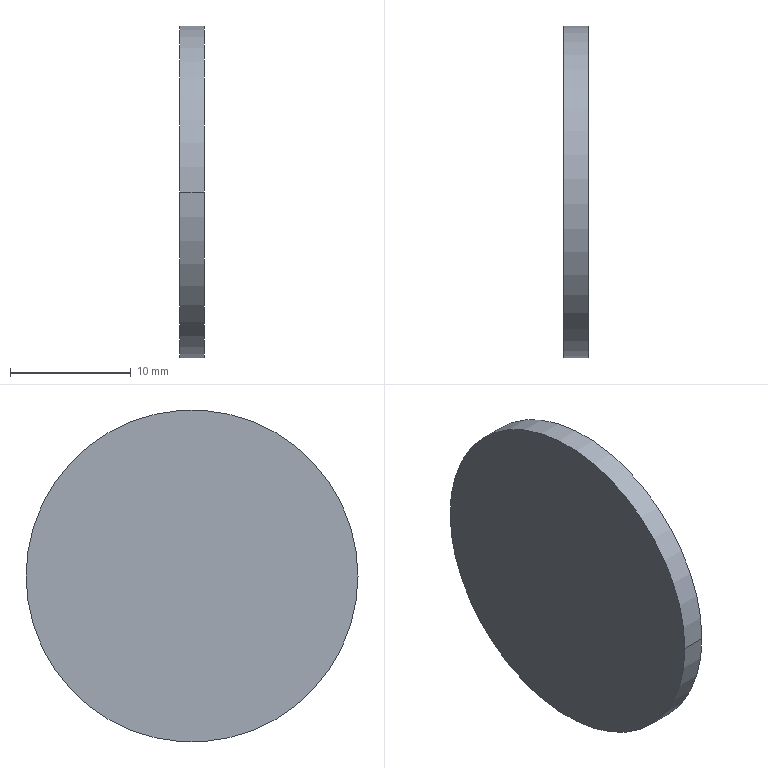Part | STEP file | 1 solid | 4 faces | box 2 x 27.5 x 27.5 mm | volume 1188 mm3 | cylinder 2 | plane 2 | commonest cylinder face diameters 27.5 x2
STEP:
#1=CARTESIAN_POINT('',(0.,0.,0.));
#2=DIRECTION('',(0.,0.,1.));
#3=DIRECTION('',(1.,0.,0.));
#4=AXIS2_PLACEMENT_3D('',#1,#2,#3);
#5=CARTESIAN_POINT('',(-24.,-13.75,0.));
#6=VERTEX_POINT('',#5);
#7=CARTESIAN_POINT('',(-22.,-13.75,0.));
#8=VERTEX_POINT('',#7);
#9=CARTESIAN_POINT('',(-24.,-13.75,0.));
#10=DIRECTION('',(1.,0.,0.));
#11=VECTOR('',#10,1.);
#12=LINE('',#9,#11);
#13=CARTESIAN_POINT('',(-24.,0.,0.));
#14=DIRECTION('',(1.,0.,0.));
#15=DIRECTION('',(0.,1.,0.));
#16=AXIS2_PLACEMENT_3D('',#13,#14,#15);
#17=CYLINDRICAL_SURFACE('',#16,13.75);
#18=CARTESIAN_POINT('',(3.142,0.));
#19=DIRECTION('',(0.,1.));
#20=VECTOR('',#19,1.);
#21=LINE('',#18,#20);
#22=(GEOMETRIC_REPRESENTATION_CONTEXT(2)PARAMETRIC_REPRESENTATION_CONTEXT()REPRESENTATION_CONTEXT('',''));
#23=DEFINITIONAL_REPRESENTATION('',(#21),#22);
#24=PCURVE('',#17,#23);
#25=CARTESIAN_POINT('',(-24.,0.,0.));
#26=DIRECTION('',(1.,0.,0.));
#27=DIRECTION('',(0.,1.,0.));
#28=AXIS2_PLACEMENT_3D('',#25,#26,#27);
#29=CYLINDRICAL_SURFACE('',#28,13.75);
#30=CARTESIAN_POINT('',(3.142,0.));
#31=DIRECTION('',(0.,1.));
#32=VECTOR('',#31,1.);
#33=LINE('',#30,#32);
#34=(GEOMETRIC_REPRESENTATION_CONTEXT(2)PARAMETRIC_REPRESENTATION_CONTEXT()REPRESENTATION_CONTEXT('',''));
#35=DEFINITIONAL_REPRESENTATION('',(#33),#34);
#36=PCURVE('',#29,#35);
#37=SURFACE_CURVE('',#12,(#24,#36),.PCURVE_S1.);
#38=EDGE_CURVE('',#6,#8,#37,.T.);
#39=ORIENTED_EDGE('',*,*,#38,.T.);
#40=CARTESIAN_POINT('',(-22.,13.75,0.));
#41=VERTEX_POINT('',#40);
#42=CARTESIAN_POINT('',(-22.,0.,0.));
#43=DIRECTION('',(1.,0.,0.));
#44=DIRECTION('',(0.,1.,0.));
#45=AXIS2_PLACEMENT_3D('',#42,#43,#44);
#46=CIRCLE('',#45,13.75);
#47=CARTESIAN_POINT('',(0.,2.));
#48=DIRECTION('',(1.,0.));
#49=VECTOR('',#48,1.);
#50=LINE('',#47,#49);
#51=(GEOMETRIC_REPRESENTATION_CONTEXT(2)PARAMETRIC_REPRESENTATION_CONTEXT()REPRESENTATION_CONTEXT('',''));
#52=DEFINITIONAL_REPRESENTATION('',(#50),#51);
#53=PCURVE('',#17,#52);
#54=CARTESIAN_POINT('',(-22.,0.,0.));
#55=DIRECTION('',(1.,0.,0.));
#56=DIRECTION('',(0.,0.,-1.));
#57=AXIS2_PLACEMENT_3D('',#54,#55,#56);
#58=PLANE('',#57);
#59=CARTESIAN_POINT('',(0.,0.));
#60=DIRECTION('',(0.,1.));
#61=AXIS2_PLACEMENT_2D('',#59,#60);
#62=CIRCLE('',#61,13.75);
#63=(GEOMETRIC_REPRESENTATION_CONTEXT(2)PARAMETRIC_REPRESENTATION_CONTEXT()REPRESENTATION_CONTEXT('',''));
#64=DEFINITIONAL_REPRESENTATION('',(#62),#63);
#65=PCURVE('',#58,#64);
#66=SURFACE_CURVE('',#46,(#53,#65),.PCURVE_S1.);
#67=EDGE_CURVE('',#41,#8,#66,.T.);
#68=ORIENTED_EDGE('',*,*,#67,.F.);
#69=CARTESIAN_POINT('',(-24.,13.75,0.));
#70=VERTEX_POINT('',#69);
#71=CARTESIAN_POINT('',(-24.,13.75,0.));
#72=DIRECTION('',(1.,0.,0.));
#73=VECTOR('',#72,1.);
#74=LINE('',#71,#73);
#75=CARTESIAN_POINT('',(0.,0.));
#76=DIRECTION('',(0.,1.));
#77=VECTOR('',#76,1.);
#78=LINE('',#75,#77);
#79=(GEOMETRIC_REPRESENTATION_CONTEXT(2)PARAMETRIC_REPRESENTATION_CONTEXT()REPRESENTATION_CONTEXT('',''));
#80=DEFINITIONAL_REPRESENTATION('',(#78),#79);
#81=PCURVE('',#17,#80);
#82=CARTESIAN_POINT('',(6.283,0.));
#83=DIRECTION('',(0.,1.));
#84=VECTOR('',#83,1.);
#85=LINE('',#82,#84);
#86=(GEOMETRIC_REPRESENTATION_CONTEXT(2)PARAMETRIC_REPRESENTATION_CONTEXT()REPRESENTATION_CONTEXT('',''));
#87=DEFINITIONAL_REPRESENTATION('',(#85),#86);
#88=PCURVE('',#29,#87);
#89=SURFACE_CURVE('',#74,(#81,#88),.PCURVE_S1.);
#90=EDGE_CURVE('',#70,#41,#89,.T.);
#91=ORIENTED_EDGE('',*,*,#90,.F.);
#92=CARTESIAN_POINT('',(-24.,0.,0.));
#93=DIRECTION('',(-1.,0.,0.));
#94=DIRECTION('',(0.,-1.,0.));
#95=AXIS2_PLACEMENT_3D('',#92,#93,#94);
#96=CIRCLE('',#95,13.75);
#97=CARTESIAN_POINT('',(3.142,0.));
#98=DIRECTION('',(-1.,0.));
#99=VECTOR('',#98,1.);
#100=LINE('',#97,#99);
#101=(GEOMETRIC_REPRESENTATION_CONTEXT(2)PARAMETRIC_REPRESENTATION_CONTEXT()REPRESENTATION_CONTEXT('',''));
#102=DEFINITIONAL_REPRESENTATION('',(#100),#101);
#103=PCURVE('',#17,#102);
#104=CARTESIAN_POINT('',(-24.,0.,0.));
#105=DIRECTION('',(1.,0.,0.));
#106=DIRECTION('',(0.,0.,-1.));
#107=AXIS2_PLACEMENT_3D('',#104,#105,#106);
#108=PLANE('',#107);
#109=CARTESIAN_POINT('',(0.,-13.75));
#110=CARTESIAN_POINT('',(-23.816,-13.75));
#111=CARTESIAN_POINT('',(-11.908,6.875));
#112=CARTESIAN_POINT('',(0.,27.5));
#113=CARTESIAN_POINT('',(11.908,6.875));
#114=CARTESIAN_POINT('',(23.816,-13.75));
#115=CARTESIAN_POINT('',(0.,-13.75));
#116=(BOUNDED_CURVE()B_SPLINE_CURVE(2,(#109,#110,#111,#112,#113,#114,#115),.UNSPECIFIED.,.T.,.F.)B_SPLINE_CURVE_WITH_KNOTS((1,2,2,2,2,1),(-2.094,0.,2.094,4.189,6.283,8.378),.UNSPECIFIED.)CURVE()GEOMETRIC_REPRESENTATION_ITEM()RATIONAL_B_SPLINE_CURVE((1.,0.5,1.,0.5,1.,0.5,1.))REPRESENTATION_ITEM(''));
#117=(GEOMETRIC_REPRESENTATION_CONTEXT(2)PARAMETRIC_REPRESENTATION_CONTEXT()REPRESENTATION_CONTEXT('',''));
#118=DEFINITIONAL_REPRESENTATION('',(#116),#117);
#119=PCURVE('',#108,#118);
#120=SURFACE_CURVE('',#96,(#103,#119),.PCURVE_S1.);
#121=EDGE_CURVE('',#6,#70,#120,.T.);
#122=ORIENTED_EDGE('',*,*,#121,.F.);
#123=EDGE_LOOP('',(#39,#68,#91,#122));
#124=FACE_BOUND('',#123,.T.);
#125=ADVANCED_FACE('',(#124),#17,.T.);
#126=CARTESIAN_POINT('',(-24.,0.,0.));
#127=DIRECTION('',(-1.,0.,0.));
#128=DIRECTION('',(0.,1.,0.));
#129=AXIS2_PLACEMENT_3D('',#126,#127,#128);
#130=CIRCLE('',#129,13.75);
#131=CARTESIAN_POINT('',(0.,13.75));
#132=CARTESIAN_POINT('',(23.816,13.75));
#133=CARTESIAN_POINT('',(11.908,-6.875));
#134=CARTESIAN_POINT('',(0.,-27.5));
#135=CARTESIAN_POINT('',(-11.908,-6.875));
#136=CARTESIAN_POINT('',(-23.816,13.75));
#137=CARTESIAN_POINT('',(0.,13.75));
#138=(BOUNDED_CURVE()B_SPLINE_CURVE(2,(#131,#132,#133,#134,#135,#136,#137),.UNSPECIFIED.,.T.,.F.)B_SPLINE_CURVE_WITH_KNOTS((1,2,2,2,2,1),(-2.094,0.,2.094,4.189,6.283,8.378),.UNSPECIFIED.)CURVE()GEOMETRIC_REPRESENTATION_ITEM()RATIONAL_B_SPLINE_CURVE((1.,0.5,1.,0.5,1.,0.5,1.))REPRESENTATION_ITEM(''));
#139=(GEOMETRIC_REPRESENTATION_CONTEXT(2)PARAMETRIC_REPRESENTATION_CONTEXT()REPRESENTATION_CONTEXT('',''));
#140=DEFINITIONAL_REPRESENTATION('',(#138),#139);
#141=PCURVE('',#108,#140);
#142=CARTESIAN_POINT('',(6.283,0.));
#143=DIRECTION('',(-1.,0.));
#144=VECTOR('',#143,1.);
#145=LINE('',#142,#144);
#146=(GEOMETRIC_REPRESENTATION_CONTEXT(2)PARAMETRIC_REPRESENTATION_CONTEXT()REPRESENTATION_CONTEXT('',''));
#147=DEFINITIONAL_REPRESENTATION('',(#145),#146);
#148=PCURVE('',#29,#147);
#149=SURFACE_CURVE('',#130,(#141,#148),.PCURVE_S1.);
#150=EDGE_CURVE('',#70,#6,#149,.T.);
#151=ORIENTED_EDGE('',*,*,#150,.F.);
#152=ORIENTED_EDGE('',*,*,#121,.F.);
#153=EDGE_LOOP('',(#151,#152));
#154=FACE_BOUND('',#153,.F.);
#155=ADVANCED_FACE('',(#154),#108,.F.);
#156=ORIENTED_EDGE('',*,*,#90,.T.);
#157=CARTESIAN_POINT('',(-22.,0.,0.));
#158=DIRECTION('',(1.,0.,0.));
#159=DIRECTION('',(0.,-1.,0.));
#160=AXIS2_PLACEMENT_3D('',#157,#158,#159);
#161=CIRCLE('',#160,13.75);
#162=CARTESIAN_POINT('',(3.142,2.));
#163=DIRECTION('',(1.,0.));
#164=VECTOR('',#163,1.);
#165=LINE('',#162,#164);
#166=(GEOMETRIC_REPRESENTATION_CONTEXT(2)PARAMETRIC_REPRESENTATION_CONTEXT()REPRESENTATION_CONTEXT('',''));
#167=DEFINITIONAL_REPRESENTATION('',(#165),#166);
#168=PCURVE('',#29,#167);
#169=CARTESIAN_POINT('',(0.,0.));
#170=DIRECTION('',(0.,-1.));
#171=AXIS2_PLACEMENT_2D('',#169,#170);
#172=CIRCLE('',#171,13.75);
#173=(GEOMETRIC_REPRESENTATION_CONTEXT(2)PARAMETRIC_REPRESENTATION_CONTEXT()REPRESENTATION_CONTEXT('',''));
#174=DEFINITIONAL_REPRESENTATION('',(#172),#173);
#175=PCURVE('',#58,#174);
#176=SURFACE_CURVE('',#161,(#168,#175),.PCURVE_S1.);
#177=EDGE_CURVE('',#8,#41,#176,.T.);
#178=ORIENTED_EDGE('',*,*,#177,.F.);
#179=ORIENTED_EDGE('',*,*,#38,.F.);
#180=ORIENTED_EDGE('',*,*,#150,.F.);
#181=EDGE_LOOP('',(#156,#178,#179,#180));
#182=FACE_BOUND('',#181,.T.);
#183=ADVANCED_FACE('',(#182),#29,.T.);
#184=ORIENTED_EDGE('',*,*,#177,.F.);
#185=ORIENTED_EDGE('',*,*,#67,.F.);
#186=EDGE_LOOP('',(#184,#185));
#187=FACE_BOUND('',#186,.F.);
#188=ADVANCED_FACE('',(#187),#58,.T.);
#189=CLOSED_SHELL('',(#125,#155,#183,#188));
#190=MANIFOLD_SOLID_BREP('',#189);
#191=(LENGTH_UNIT()NAMED_UNIT(*)SI_UNIT(.MILLI.,.METRE.));
#192=UNCERTAINTY_MEASURE_WITH_UNIT(LENGTH_MEASURE(0.0000001),#191,'','');
#193=(NAMED_UNIT(*)PLANE_ANGLE_UNIT()SI_UNIT($,.RADIAN.));
#194=(NAMED_UNIT(*)SI_UNIT($,.STERADIAN.)SOLID_ANGLE_UNIT());
#195=(GEOMETRIC_REPRESENTATION_CONTEXT(3)GLOBAL_UNCERTAINTY_ASSIGNED_CONTEXT((#192))GLOBAL_UNIT_ASSIGNED_CONTEXT((#191,#193,#194))REPRESENTATION_CONTEXT('',''));
#196=ADVANCED_BREP_SHAPE_REPRESENTATION('',(#4,#190),#195);